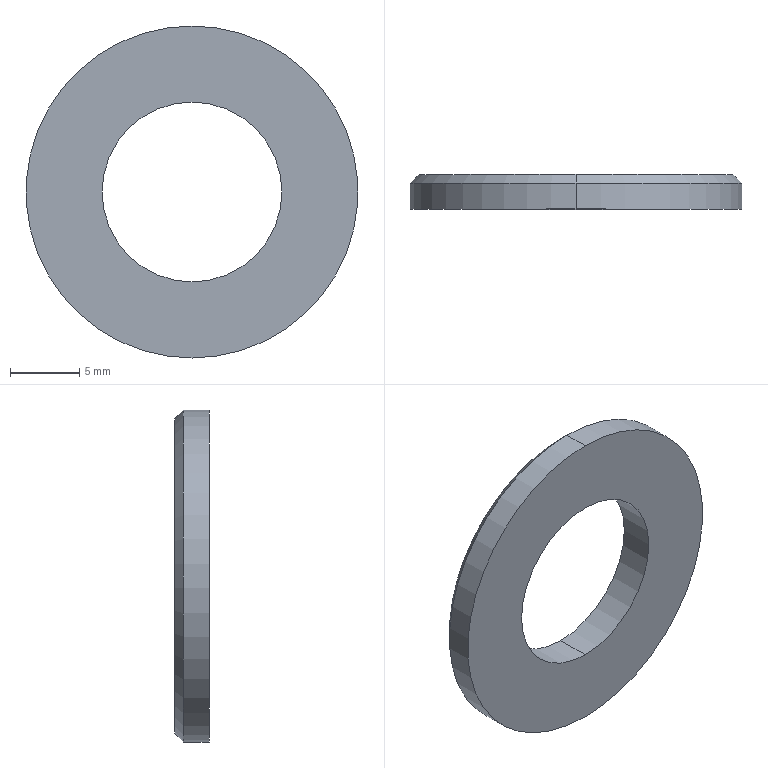Part | SolidWorks | 1 solid | 8 faces | box 24 x 2.5 x 24 mm | volume 784.672 mm3 | cylinder 4 | cone 2 | plane 2 | commonest cylinder face diameters 13 x2 24 x2
STEP:
#1=CARTESIAN_POINT('',(0.,10.52,-12.));
#2=VERTEX_POINT('',#1);
#3=CARTESIAN_POINT('',(0.,10.52,12.));
#4=VERTEX_POINT('',#3);
#5=CARTESIAN_POINT('',(0.,10.52,0.));
#6=DIRECTION('',(0.,-1.,0.));
#7=DIRECTION('',(0.,0.,-1.));
#8=AXIS2_PLACEMENT_3D('',#5,#6,#7);
#9=CIRCLE('',#8,12.);
#10=EDGE_CURVE('',#2,#4,#9,.T.);
#11=ORIENTED_EDGE('',*,*,#10,.T.);
#12=CARTESIAN_POINT('',(0.,8.645,12.));
#13=VERTEX_POINT('',#12);
#14=CARTESIAN_POINT('',(0.,0.,12.));
#15=DIRECTION('',(0.,-1.,0.));
#16=VECTOR('',#15,1000.);
#17=LINE('',#14,#16);
#18=EDGE_CURVE('',#4,#13,#17,.T.);
#19=ORIENTED_EDGE('',*,*,#18,.T.);
#20=CARTESIAN_POINT('',(0.,8.645,-12.));
#21=VERTEX_POINT('',#20);
#22=CARTESIAN_POINT('',(0.,8.645,0.));
#23=DIRECTION('',(0.,-1.,0.));
#24=DIRECTION('',(0.,0.,-1.));
#25=AXIS2_PLACEMENT_3D('',#22,#23,#24);
#26=CIRCLE('',#25,12.);
#27=EDGE_CURVE('',#21,#13,#26,.T.);
#28=ORIENTED_EDGE('',*,*,#27,.F.);
#29=CARTESIAN_POINT('',(0.,0.,-12.));
#30=DIRECTION('',(0.,-1.,0.));
#31=VECTOR('',#30,1000.);
#32=LINE('',#29,#31);
#33=EDGE_CURVE('',#2,#21,#32,.T.);
#34=ORIENTED_EDGE('',*,*,#33,.F.);
#35=EDGE_LOOP('',(#11,#19,#28,#34));
#36=FACE_OUTER_BOUND('',#35,.T.);
#37=CARTESIAN_POINT('',(0.,0.,0.));
#38=DIRECTION('',(0.,-1.,0.));
#39=DIRECTION('',(0.,0.,-1.));
#40=AXIS2_PLACEMENT_3D('',#37,#38,#39);
#41=CYLINDRICAL_SURFACE('',#40,12.);
#42=ADVANCED_FACE('',(#36),#41,.T.);
#43=CARTESIAN_POINT('',(0.,11.145,-11.375));
#44=VERTEX_POINT('',#43);
#45=CARTESIAN_POINT('',(0.,11.145,11.375));
#46=VERTEX_POINT('',#45);
#47=CARTESIAN_POINT('',(0.,11.145,0.));
#48=DIRECTION('',(0.,-1.,0.));
#49=DIRECTION('',(0.,0.,-1.));
#50=AXIS2_PLACEMENT_3D('',#47,#48,#49);
#51=CIRCLE('',#50,11.375);
#52=EDGE_CURVE('',#44,#46,#51,.T.);
#53=ORIENTED_EDGE('',*,*,#52,.T.);
#54=CARTESIAN_POINT('',(0.,11.145,11.375));
#55=DIRECTION('',(0.,-0.7071,0.7071));
#56=VECTOR('',#55,1000.);
#57=LINE('',#54,#56);
#58=EDGE_CURVE('',#46,#4,#57,.T.);
#59=ORIENTED_EDGE('',*,*,#58,.T.);
#60=ORIENTED_EDGE('',*,*,#10,.F.);
#61=CARTESIAN_POINT('',(0.,11.145,-11.375));
#62=DIRECTION('',(0.,-0.7071,-0.7071));
#63=VECTOR('',#62,1000.);
#64=LINE('',#61,#63);
#65=EDGE_CURVE('',#44,#2,#64,.T.);
#66=ORIENTED_EDGE('',*,*,#65,.F.);
#67=EDGE_LOOP('',(#53,#59,#60,#66));
#68=FACE_OUTER_BOUND('',#67,.T.);
#69=CARTESIAN_POINT('',(0.,11.145,0.));
#70=DIRECTION('',(0.,-1.,0.));
#71=DIRECTION('',(0.,0.,-1.));
#72=AXIS2_PLACEMENT_3D('',#69,#70,#71);
#73=CONICAL_SURFACE('',#72,11.375,0.7854);
#74=ADVANCED_FACE('',(#68),#73,.T.);
#75=CARTESIAN_POINT('',(0.,11.145,6.5));
#76=VERTEX_POINT('',#75);
#77=CARTESIAN_POINT('',(0.,11.145,-6.5));
#78=VERTEX_POINT('',#77);
#79=CARTESIAN_POINT('',(0.,11.145,0.));
#80=DIRECTION('',(0.,-1.,0.));
#81=DIRECTION('',(0.,0.,-1.));
#82=AXIS2_PLACEMENT_3D('',#79,#80,#81);
#83=CIRCLE('',#82,6.5);
#84=EDGE_CURVE('',#76,#78,#83,.T.);
#85=ORIENTED_EDGE('',*,*,#84,.F.);
#86=CARTESIAN_POINT('',(0.,8.645,6.5));
#87=VERTEX_POINT('',#86);
#88=CARTESIAN_POINT('',(0.,0.,6.5));
#89=DIRECTION('',(0.,-1.,0.));
#90=VECTOR('',#89,1000.);
#91=LINE('',#88,#90);
#92=EDGE_CURVE('',#76,#87,#91,.T.);
#93=ORIENTED_EDGE('',*,*,#92,.T.);
#94=CARTESIAN_POINT('',(0.,8.645,-6.5));
#95=VERTEX_POINT('',#94);
#96=CARTESIAN_POINT('',(0.,8.645,0.));
#97=DIRECTION('',(0.,-1.,0.));
#98=DIRECTION('',(0.,0.,-1.));
#99=AXIS2_PLACEMENT_3D('',#96,#97,#98);
#100=CIRCLE('',#99,6.5);
#101=EDGE_CURVE('',#87,#95,#100,.T.);
#102=ORIENTED_EDGE('',*,*,#101,.T.);
#103=CARTESIAN_POINT('',(0.,0.,-6.5));
#104=DIRECTION('',(0.,-1.,0.));
#105=VECTOR('',#104,1000.);
#106=LINE('',#103,#105);
#107=EDGE_CURVE('',#78,#95,#106,.T.);
#108=ORIENTED_EDGE('',*,*,#107,.F.);
#109=EDGE_LOOP('',(#85,#93,#102,#108));
#110=FACE_OUTER_BOUND('',#109,.T.);
#111=CARTESIAN_POINT('',(0.,0.,0.));
#112=DIRECTION('',(0.,-1.,0.));
#113=DIRECTION('',(0.,0.,-1.));
#114=AXIS2_PLACEMENT_3D('',#111,#112,#113);
#115=CYLINDRICAL_SURFACE('',#114,6.5);
#116=ADVANCED_FACE('',(#110),#115,.F.);
#117=ORIENTED_EDGE('',*,*,#92,.F.);
#118=CARTESIAN_POINT('',(0.,11.145,0.));
#119=DIRECTION('',(0.,-1.,0.));
#120=DIRECTION('',(0.,0.,-1.));
#121=AXIS2_PLACEMENT_3D('',#118,#119,#120);
#122=CIRCLE('',#121,6.5);
#123=EDGE_CURVE('',#78,#76,#122,.T.);
#124=ORIENTED_EDGE('',*,*,#123,.F.);
#125=ORIENTED_EDGE('',*,*,#107,.T.);
#126=CARTESIAN_POINT('',(0.,8.645,0.));
#127=DIRECTION('',(0.,-1.,0.));
#128=DIRECTION('',(0.,0.,-1.));
#129=AXIS2_PLACEMENT_3D('',#126,#127,#128);
#130=CIRCLE('',#129,6.5);
#131=EDGE_CURVE('',#95,#87,#130,.T.);
#132=ORIENTED_EDGE('',*,*,#131,.T.);
#133=EDGE_LOOP('',(#117,#124,#125,#132));
#134=FACE_OUTER_BOUND('',#133,.T.);
#135=CARTESIAN_POINT('',(0.,0.,0.));
#136=DIRECTION('',(0.,-1.,0.));
#137=DIRECTION('',(0.,0.,-1.));
#138=AXIS2_PLACEMENT_3D('',#135,#136,#137);
#139=CYLINDRICAL_SURFACE('',#138,6.5);
#140=ADVANCED_FACE('',(#134),#139,.F.);
#141=ORIENTED_EDGE('',*,*,#52,.F.);
#142=CARTESIAN_POINT('',(0.,11.145,0.));
#143=DIRECTION('',(0.,-1.,0.));
#144=DIRECTION('',(0.,0.,-1.));
#145=AXIS2_PLACEMENT_3D('',#142,#143,#144);
#146=CIRCLE('',#145,11.375);
#147=EDGE_CURVE('',#46,#44,#146,.T.);
#148=ORIENTED_EDGE('',*,*,#147,.F.);
#149=EDGE_LOOP('',(#141,#148));
#150=FACE_OUTER_BOUND('',#149,.T.);
#151=ORIENTED_EDGE('',*,*,#123,.T.);
#152=ORIENTED_EDGE('',*,*,#84,.T.);
#153=EDGE_LOOP('',(#151,#152));
#154=FACE_BOUND('',#153,.T.);
#155=CARTESIAN_POINT('',(-6.5,11.145,0.));
#156=DIRECTION('',(0.,-1.,0.));
#157=DIRECTION('',(0.,0.,-1.));
#158=AXIS2_PLACEMENT_3D('',#155,#156,#157);
#159=PLANE('',#158);
#160=ADVANCED_FACE('',(#150,#154),#159,.F.);
#161=ORIENTED_EDGE('',*,*,#58,.F.);
#162=ORIENTED_EDGE('',*,*,#147,.T.);
#163=ORIENTED_EDGE('',*,*,#65,.T.);
#164=CARTESIAN_POINT('',(0.,10.52,0.));
#165=DIRECTION('',(0.,-1.,0.));
#166=DIRECTION('',(0.,0.,-1.));
#167=AXIS2_PLACEMENT_3D('',#164,#165,#166);
#168=CIRCLE('',#167,12.);
#169=EDGE_CURVE('',#4,#2,#168,.T.);
#170=ORIENTED_EDGE('',*,*,#169,.F.);
#171=EDGE_LOOP('',(#161,#162,#163,#170));
#172=FACE_OUTER_BOUND('',#171,.T.);
#173=CARTESIAN_POINT('',(0.,11.145,0.));
#174=DIRECTION('',(0.,-1.,0.));
#175=DIRECTION('',(0.,0.,-1.));
#176=AXIS2_PLACEMENT_3D('',#173,#174,#175);
#177=CONICAL_SURFACE('',#176,11.375,0.7854);
#178=ADVANCED_FACE('',(#172),#177,.T.);
#179=ORIENTED_EDGE('',*,*,#18,.F.);
#180=ORIENTED_EDGE('',*,*,#169,.T.);
#181=ORIENTED_EDGE('',*,*,#33,.T.);
#182=CARTESIAN_POINT('',(0.,8.645,0.));
#183=DIRECTION('',(0.,-1.,0.));
#184=DIRECTION('',(0.,0.,-1.));
#185=AXIS2_PLACEMENT_3D('',#182,#183,#184);
#186=CIRCLE('',#185,12.);
#187=EDGE_CURVE('',#13,#21,#186,.T.);
#188=ORIENTED_EDGE('',*,*,#187,.F.);
#189=EDGE_LOOP('',(#179,#180,#181,#188));
#190=FACE_OUTER_BOUND('',#189,.T.);
#191=CARTESIAN_POINT('',(0.,0.,0.));
#192=DIRECTION('',(0.,-1.,0.));
#193=DIRECTION('',(0.,0.,-1.));
#194=AXIS2_PLACEMENT_3D('',#191,#192,#193);
#195=CYLINDRICAL_SURFACE('',#194,12.);
#196=ADVANCED_FACE('',(#190),#195,.T.);
#197=ORIENTED_EDGE('',*,*,#131,.F.);
#198=ORIENTED_EDGE('',*,*,#101,.F.);
#199=EDGE_LOOP('',(#197,#198));
#200=FACE_BOUND('',#199,.T.);
#201=ORIENTED_EDGE('',*,*,#27,.T.);
#202=ORIENTED_EDGE('',*,*,#187,.T.);
#203=EDGE_LOOP('',(#201,#202));
#204=FACE_OUTER_BOUND('',#203,.T.);
#205=CARTESIAN_POINT('',(-6.5,8.645,0.));
#206=DIRECTION('',(0.,1.,0.));
#207=DIRECTION('',(0.,0.,1.));
#208=AXIS2_PLACEMENT_3D('',#205,#206,#207);
#209=PLANE('',#208);
#210=ADVANCED_FACE('',(#200,#204),#209,.F.);
#211=CLOSED_SHELL('',(#42,#74,#116,#140,#160,#178,#196,#210));
#212=MANIFOLD_SOLID_BREP('',#211);
#213=CARTESIAN_POINT('',(0.,0.,0.));
#214=DIRECTION('',(0.,0.,1.));
#215=DIRECTION('',(1.,0.,0.));
#216=AXIS2_PLACEMENT_3D('',#213,#214,#215);
#217=(LENGTH_UNIT()NAMED_UNIT(*)SI_UNIT(.MILLI.,.METRE.));
#218=UNCERTAINTY_MEASURE_WITH_UNIT(LENGTH_MEASURE(0.00001),#217,'','');
#219=(NAMED_UNIT(*)PLANE_ANGLE_UNIT()SI_UNIT($,.RADIAN.));
#220=(NAMED_UNIT(*)SI_UNIT($,.STERADIAN.)SOLID_ANGLE_UNIT());
#221=(GEOMETRIC_REPRESENTATION_CONTEXT(3)GLOBAL_UNCERTAINTY_ASSIGNED_CONTEXT((#218))GLOBAL_UNIT_ASSIGNED_CONTEXT((#217,#219,#220))REPRESENTATION_CONTEXT('',''));
#222=ADVANCED_BREP_SHAPE_REPRESENTATION('',(#212,#216),#221);